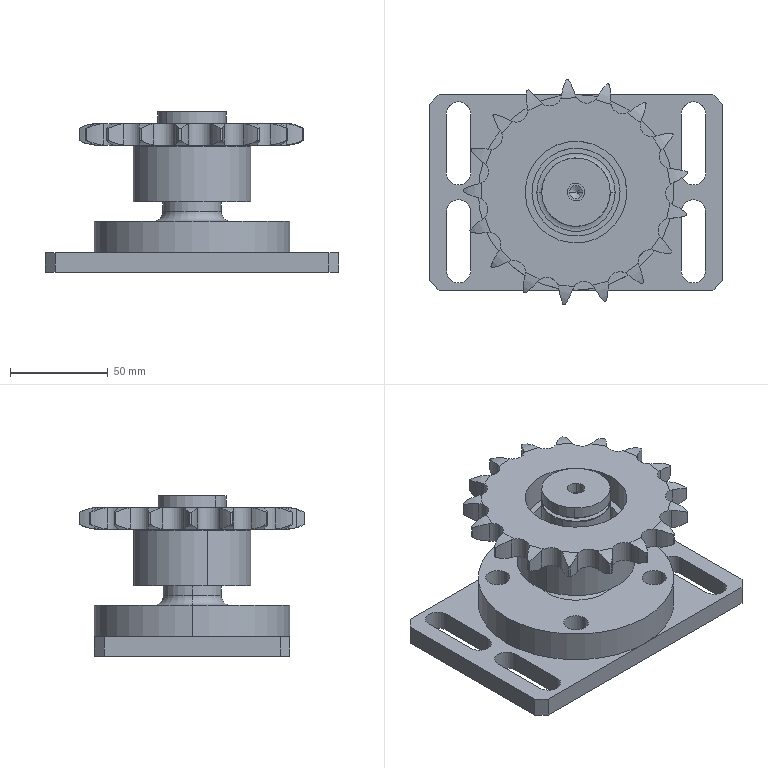Part | SolidWorks | 6 solids | 412 faces | box 150 x 115.004 x 82 mm | volume 375409 mm3 | cylinder 143 | torus 128 | sphere 68 | plane 37 | spline 34 | cone 2 | commonest cylinder face diameters 55.039 x35 12.191 x23 115.416 x17 12.5 x16 10.2 x8 23 x8